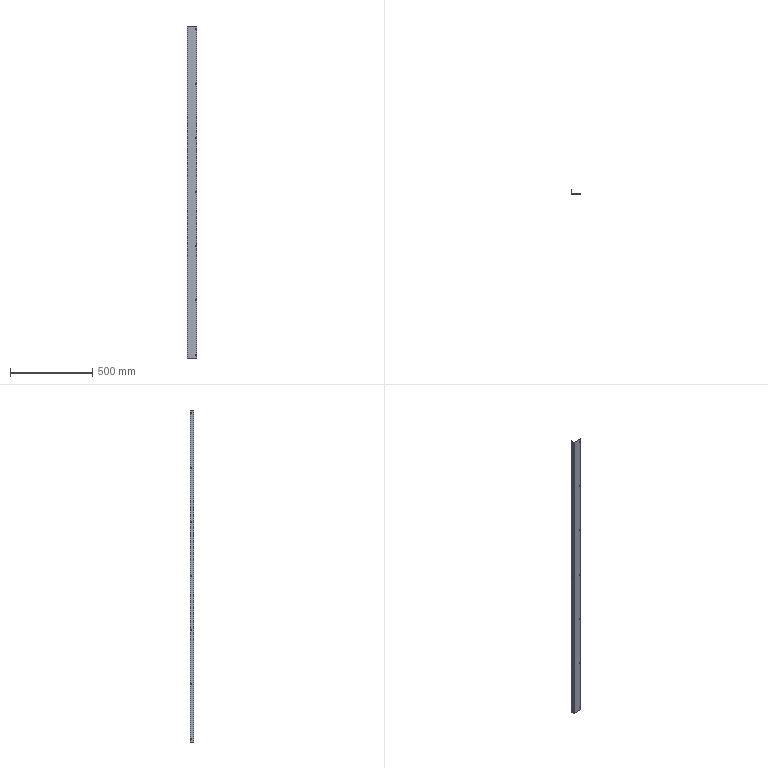Part | 1 solid | 70 faces | box 60 x 24 x 2016 mm | volume 166074 mm3 | plane 40 | cylinder 30 | commonest cylinder face diameters 6 x28 0.4 x1 2.4 x1